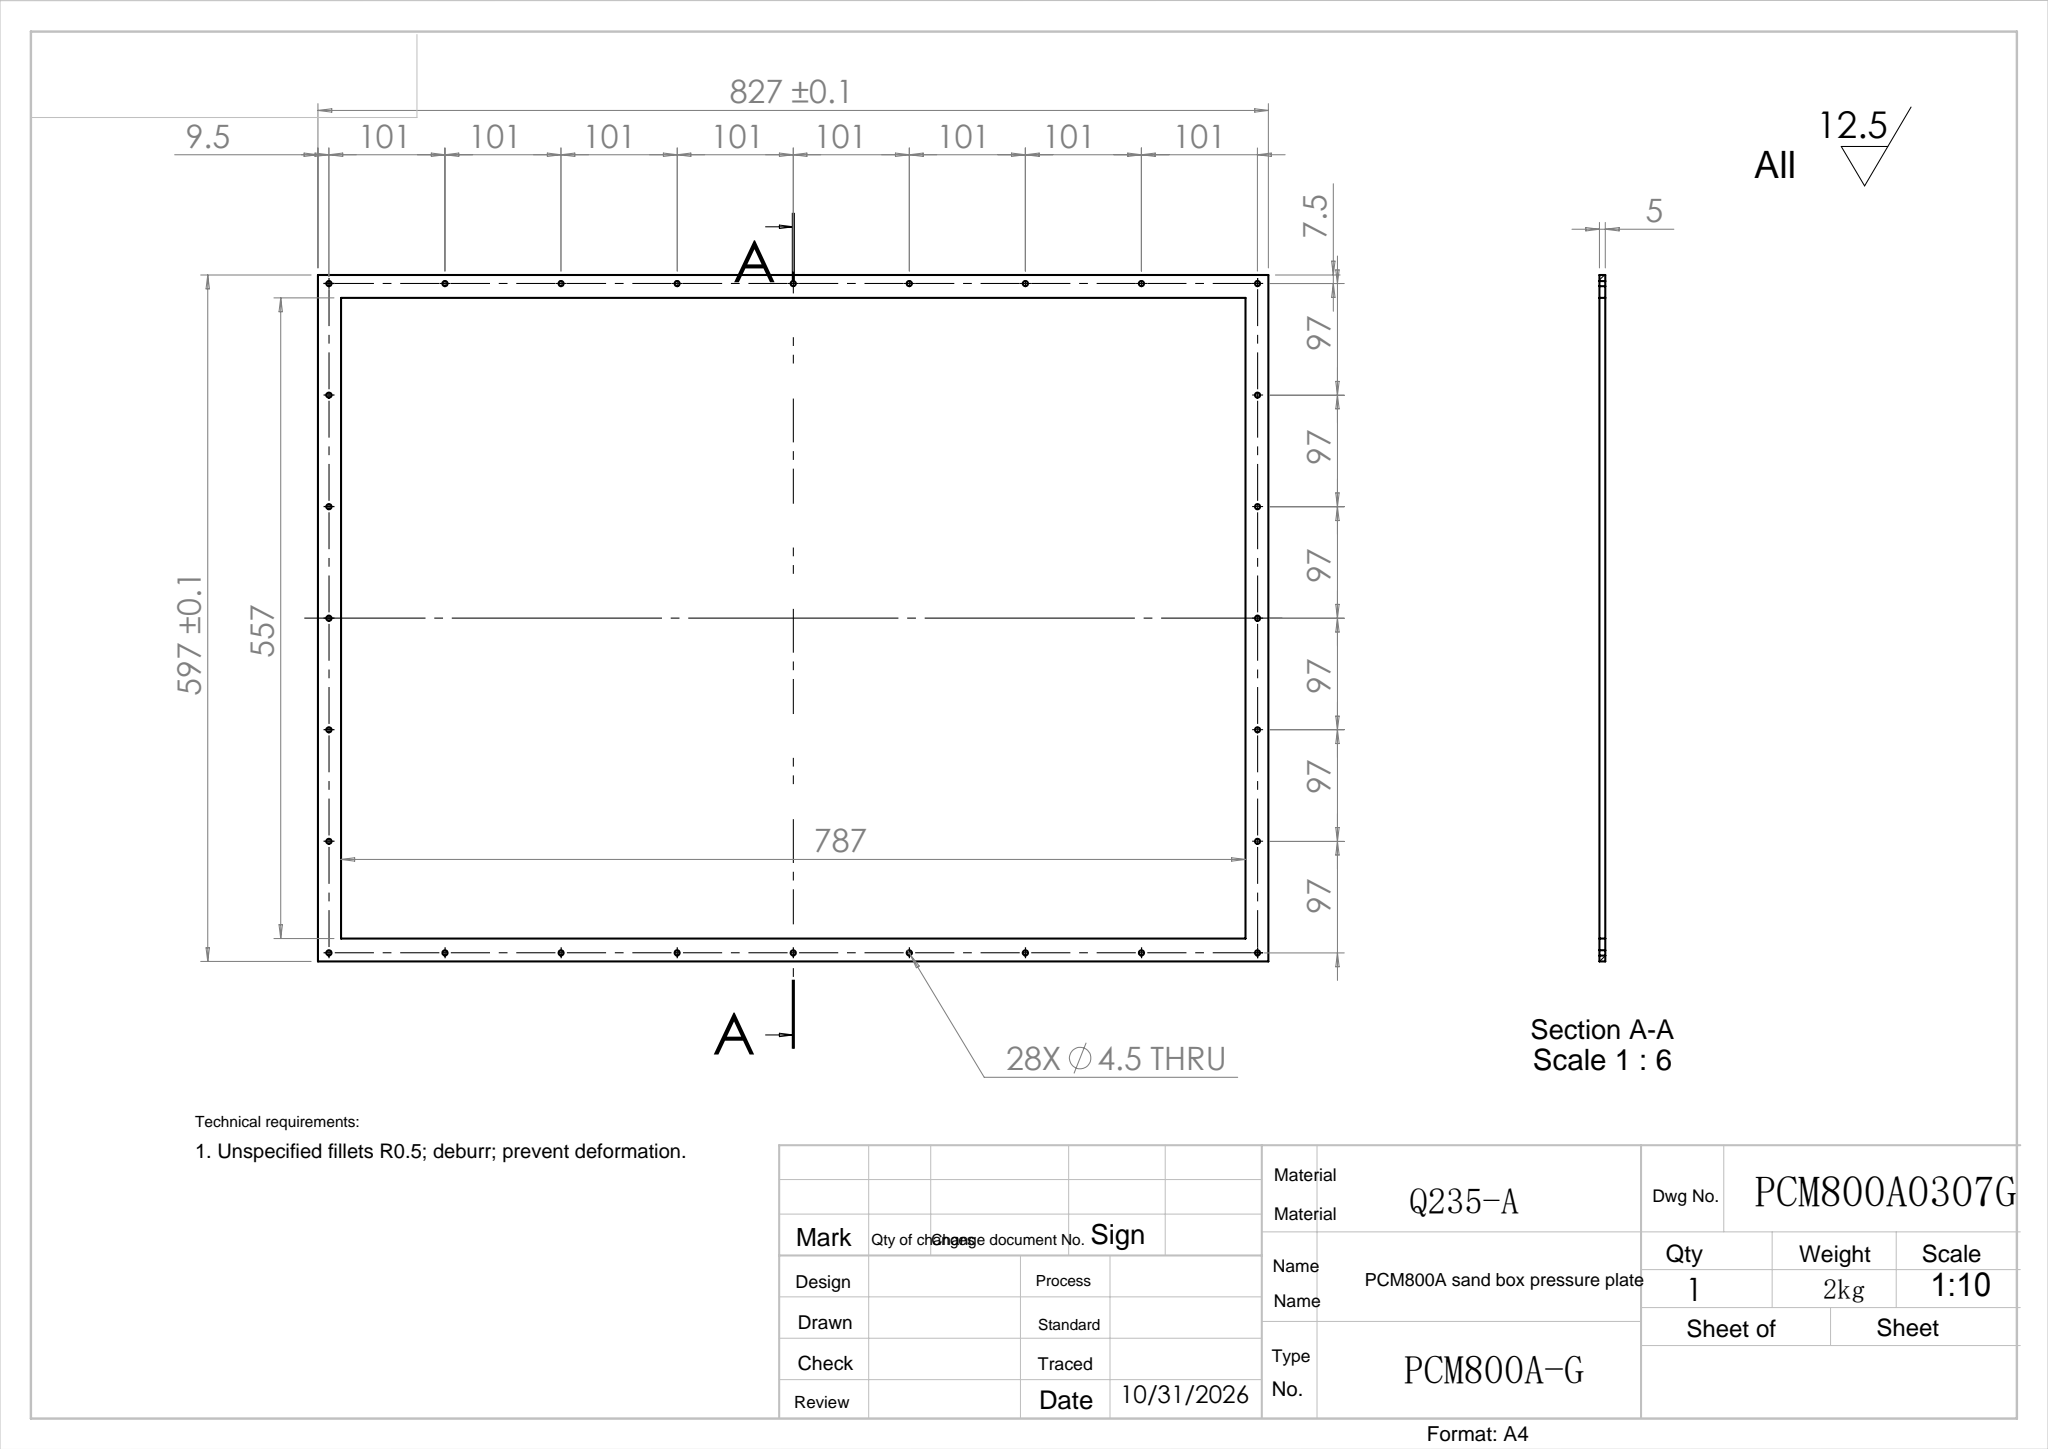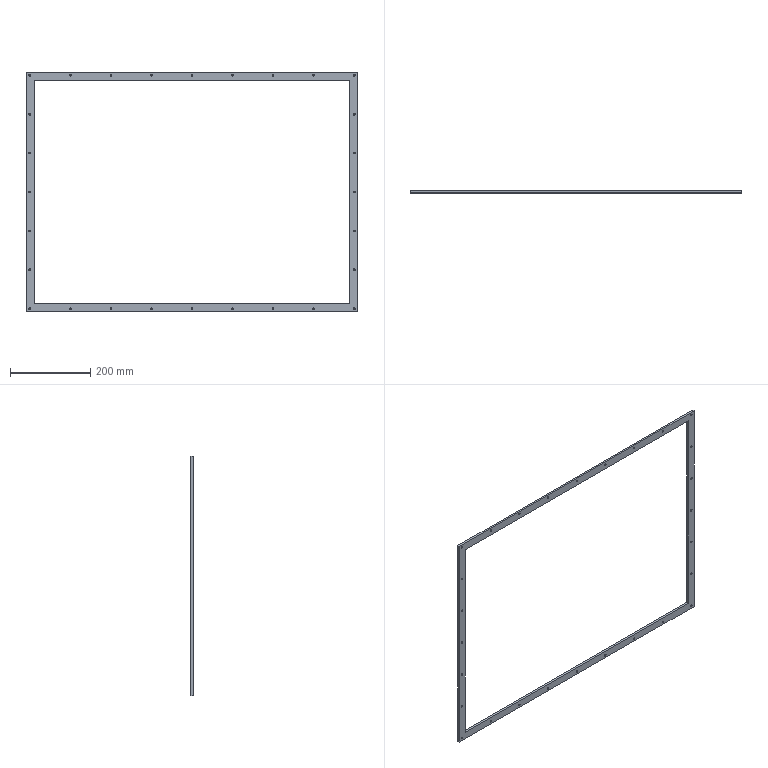Part | SolidWorks | features LPattern 3, Cut 1, Extrusion 1 | 1 solid | 66 faces | box 827 x 5 x 597 mm | volume 274573 mm3 | cylinder 56 | plane 10 | commonest cylinder face diameters 4.5 x56